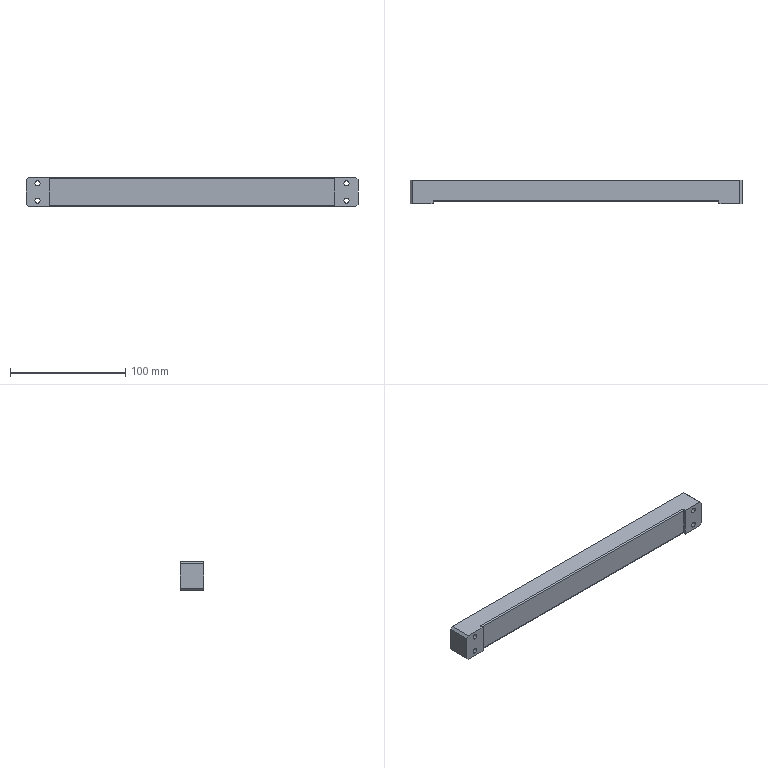Part | STEP file | 1 solid | 36 faces | box 288 x 20 x 25 mm | volume 129456 mm3 | cylinder 18 | plane 18 | commonest cylinder face diameters 4.5 x8 8 x8 2 x2